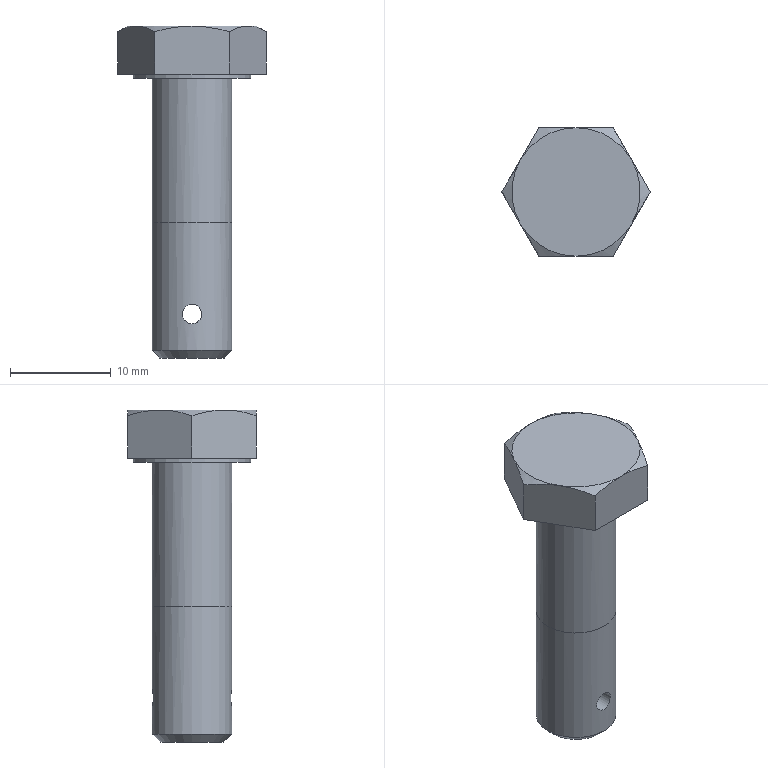Part | NX | features solid 2 | 1 solid | 21 faces | box 14.723 x 12.751 x 32.963 mm | volume 2058 mm3 | plane 10 | cone 7 | cylinder 4 | commonest cylinder face diameters 7.938 x2 1.93 x1 11.684 x1
STEP:
#1=CARTESIAN_POINT('',(0.,-3.969,-29.562));
#2=VERTEX_POINT('',#1);
#3=CARTESIAN_POINT('',(0.7571,-3.91,-29.353));
#4=CARTESIAN_POINT('',(-0.000144,-3.998,-29.667));
#5=CARTESIAN_POINT('',(-0.7565,-3.91,-29.353));
#6=CARTESIAN_POINT('',(-1.07,-3.819,-28.598));
#7=CARTESIAN_POINT('',(-0.7564,-3.91,-27.841));
#8=CARTESIAN_POINT('',(-0.0004429,-3.998,-27.528));
#9=CARTESIAN_POINT('',(0.7557,-3.91,-27.84));
#10=CARTESIAN_POINT('',(1.07,-3.819,-28.597));
#11=CARTESIAN_POINT('',(0.7571,-3.91,-29.353));
#12=CARTESIAN_POINT('',(-0.000144,-3.998,-29.667));
#13=CARTESIAN_POINT('',(-0.7565,-3.91,-29.353));
#14=B_SPLINE_CURVE_WITH_KNOTS('',3,(#3,#4,#5,#6,#7,#8,#9,#10,#11,#12,#13),.UNSPECIFIED.,.T.,.F.,(1,1,1,1,1,1,1,1,1,1,1,1,1,1,1),(-0.002271,-0.001514,-0.0007572,0.,0.0007572,0.001514,0.002271,0.003029,0.003786,0.004543,0.0053,0.006057,0.006814,0.007572,0.008329),.UNSPECIFIED.);
#15=EDGE_CURVE('',#2,#2,#14,.T.);
#16=ORIENTED_EDGE('',*,*,#15,.T.);
#17=EDGE_LOOP('',(#16));
#18=FACE_BOUND('',#17,.T.);
#19=CARTESIAN_POINT('',(-3.969,0.,-19.469));
#20=VERTEX_POINT('',#19);
#21=CARTESIAN_POINT('',(-3.11,3.11,-19.469));
#22=CARTESIAN_POINT('',(-4.398,0.,-19.469));
#23=CARTESIAN_POINT('',(-3.11,-3.11,-19.469));
#24=CARTESIAN_POINT('',(0.,-4.398,-19.469));
#25=CARTESIAN_POINT('',(3.11,-3.11,-19.469));
#26=CARTESIAN_POINT('',(4.398,0.,-19.469));
#27=CARTESIAN_POINT('',(3.11,3.11,-19.469));
#28=CARTESIAN_POINT('',(0.,4.398,-19.469));
#29=CARTESIAN_POINT('',(-3.11,3.11,-19.469));
#30=CARTESIAN_POINT('',(-4.398,0.,-19.469));
#31=CARTESIAN_POINT('',(-3.11,-3.11,-19.469));
#32=B_SPLINE_CURVE_WITH_KNOTS('',3,(#21,#22,#23,#24,#25,#26,#27,#28,#29,#30,#31),.UNSPECIFIED.,.T.,.F.,(1,1,1,1,1,1,1,1,1,1,1,1,1,1,1),(-0.375,-0.25,-0.125,0.,0.125,0.25,0.375,0.5,0.625,0.75,0.875,1.,1.125,1.25,1.375),.UNSPECIFIED.);
#33=EDGE_CURVE('',#20,#20,#32,.T.);
#34=ORIENTED_EDGE('',*,*,#33,.F.);
#35=EDGE_LOOP('',(#34));
#36=FACE_BOUND('',#35,.T.);
#37=CARTESIAN_POINT('',(-3.969,0.,-32.175));
#38=VERTEX_POINT('',#37);
#39=CARTESIAN_POINT('',(0.,0.,-32.175));
#40=DIRECTION('',(0.,0.,-1.));
#41=DIRECTION('',(-1.,0.,0.));
#42=AXIS2_PLACEMENT_3D('',#39,#40,#41);
#43=CIRCLE('',#42,3.969);
#44=EDGE_CURVE('',#38,#38,#43,.T.);
#45=ORIENTED_EDGE('',*,*,#44,.F.);
#46=EDGE_LOOP('',(#45));
#47=FACE_BOUND('',#46,.T.);
#48=CARTESIAN_POINT('',(0.,3.969,-29.562));
#49=VERTEX_POINT('',#48);
#50=CARTESIAN_POINT('',(-0.7571,3.91,-29.353));
#51=CARTESIAN_POINT('',(0.000144,3.998,-29.667));
#52=CARTESIAN_POINT('',(0.7565,3.91,-29.353));
#53=CARTESIAN_POINT('',(1.07,3.819,-28.598));
#54=CARTESIAN_POINT('',(0.7564,3.91,-27.841));
#55=CARTESIAN_POINT('',(0.0004429,3.998,-27.528));
#56=CARTESIAN_POINT('',(-0.7557,3.91,-27.84));
#57=CARTESIAN_POINT('',(-1.07,3.819,-28.597));
#58=CARTESIAN_POINT('',(-0.7571,3.91,-29.353));
#59=CARTESIAN_POINT('',(0.000144,3.998,-29.667));
#60=CARTESIAN_POINT('',(0.7565,3.91,-29.353));
#61=B_SPLINE_CURVE_WITH_KNOTS('',3,(#50,#51,#52,#53,#54,#55,#56,#57,#58,#59,#60),.UNSPECIFIED.,.T.,.F.,(1,1,1,1,1,1,1,1,1,1,1,1,1,1,1),(-0.002271,-0.001514,-0.0007572,0.,0.0007572,0.001514,0.002271,0.003029,0.003786,0.004543,0.0053,0.006057,0.006814,0.007572,0.008329),.UNSPECIFIED.);
#62=EDGE_CURVE('',#49,#49,#61,.T.);
#63=ORIENTED_EDGE('',*,*,#62,.T.);
#64=EDGE_LOOP('',(#63));
#65=FACE_BOUND('',#64,.T.);
#66=CARTESIAN_POINT('',(0.,0.,0.));
#67=DIRECTION('',(0.,0.,-1.));
#68=DIRECTION('',(-1.,0.,0.));
#69=AXIS2_PLACEMENT_3D('',#66,#67,#68);
#70=CYLINDRICAL_SURFACE('',#69,3.969);
#71=ADVANCED_FACE('',(#18,#36,#47,#65),#70,.T.);
#72=CARTESIAN_POINT('',(-3.969,0.,-5.182));
#73=VERTEX_POINT('',#72);
#74=CARTESIAN_POINT('',(0.,0.,-5.182));
#75=DIRECTION('',(0.,0.,-1.));
#76=DIRECTION('',(-1.,0.,0.));
#77=AXIS2_PLACEMENT_3D('',#74,#75,#76);
#78=CIRCLE('',#77,3.969);
#79=EDGE_CURVE('',#73,#73,#78,.T.);
#80=ORIENTED_EDGE('',*,*,#79,.T.);
#81=EDGE_LOOP('',(#80));
#82=FACE_BOUND('',#81,.T.);
#83=ORIENTED_EDGE('',*,*,#33,.T.);
#84=EDGE_LOOP('',(#83));
#85=FACE_BOUND('',#84,.T.);
#86=CARTESIAN_POINT('',(0.,0.,0.));
#87=DIRECTION('',(0.,0.,-1.));
#88=DIRECTION('',(-1.,0.,0.));
#89=AXIS2_PLACEMENT_3D('',#86,#87,#88);
#90=CYLINDRICAL_SURFACE('',#89,3.969);
#91=ADVANCED_FACE('',(#82,#85),#90,.T.);
#92=CARTESIAN_POINT('',(-7.362,0.,-4.775));
#93=VERTEX_POINT('',#92);
#94=CARTESIAN_POINT('',(-3.681,6.375,-4.775));
#95=VERTEX_POINT('',#94);
#96=CARTESIAN_POINT('',(-4.061,5.717,-4.775));
#97=DIRECTION('',(0.5,0.866,0.));
#98=VECTOR('',#97,1000.);
#99=LINE('',#96,#98);
#100=EDGE_CURVE('',#93,#95,#99,.T.);
#101=ORIENTED_EDGE('',*,*,#100,.T.);
#102=CARTESIAN_POINT('',(3.681,6.375,-4.775));
#103=VERTEX_POINT('',#102);
#104=CARTESIAN_POINT('',(5.842,6.375,-4.775));
#105=DIRECTION('',(1.,0.,0.));
#106=VECTOR('',#105,1000.);
#107=LINE('',#104,#106);
#108=EDGE_CURVE('',#95,#103,#107,.T.);
#109=ORIENTED_EDGE('',*,*,#108,.T.);
#110=CARTESIAN_POINT('',(7.362,0.,-4.775));
#111=VERTEX_POINT('',#110);
#112=CARTESIAN_POINT('',(6.982,0.658,-4.775));
#113=DIRECTION('',(0.5,-0.866,0.));
#114=VECTOR('',#113,1000.);
#115=LINE('',#112,#114);
#116=EDGE_CURVE('',#103,#111,#115,.T.);
#117=ORIENTED_EDGE('',*,*,#116,.T.);
#118=CARTESIAN_POINT('',(3.681,-6.375,-4.775));
#119=VERTEX_POINT('',#118);
#120=CARTESIAN_POINT('',(6.982,-0.658,-4.775));
#121=DIRECTION('',(-0.5,-0.866,0.));
#122=VECTOR('',#121,1000.);
#123=LINE('',#120,#122);
#124=EDGE_CURVE('',#111,#119,#123,.T.);
#125=ORIENTED_EDGE('',*,*,#124,.T.);
#126=CARTESIAN_POINT('',(-3.681,-6.375,-4.775));
#127=VERTEX_POINT('',#126);
#128=CARTESIAN_POINT('',(5.842,-6.375,-4.775));
#129=DIRECTION('',(-1.,0.,0.));
#130=VECTOR('',#129,1000.);
#131=LINE('',#128,#130);
#132=EDGE_CURVE('',#119,#127,#131,.T.);
#133=ORIENTED_EDGE('',*,*,#132,.T.);
#134=CARTESIAN_POINT('',(-4.061,-5.717,-4.775));
#135=DIRECTION('',(-0.5,0.866,0.));
#136=VECTOR('',#135,1000.);
#137=LINE('',#134,#136);
#138=EDGE_CURVE('',#127,#93,#137,.T.);
#139=ORIENTED_EDGE('',*,*,#138,.T.);
#140=EDGE_LOOP('',(#101,#109,#117,#125,#133,#139));
#141=FACE_BOUND('',#140,.T.);
#142=CARTESIAN_POINT('',(-5.842,0.,-4.775));
#143=VERTEX_POINT('',#142);
#144=CARTESIAN_POINT('',(0.,0.,-4.775));
#145=DIRECTION('',(0.,0.,-1.));
#146=DIRECTION('',(-1.,0.,0.));
#147=AXIS2_PLACEMENT_3D('',#144,#145,#146);
#148=CIRCLE('',#147,5.842);
#149=EDGE_CURVE('',#143,#143,#148,.T.);
#150=ORIENTED_EDGE('',*,*,#149,.F.);
#151=EDGE_LOOP('',(#150));
#152=FACE_BOUND('',#151,.T.);
#153=CARTESIAN_POINT('',(5.842,0.,-4.775));
#154=DIRECTION('',(0.,0.,-1.));
#155=DIRECTION('',(-1.,0.,0.));
#156=AXIS2_PLACEMENT_3D('',#153,#154,#155);
#157=PLANE('',#156);
#158=ADVANCED_FACE('',(#141,#152),#157,.T.);
#159=CARTESIAN_POINT('',(-3.181,0.,-32.963));
#160=VERTEX_POINT('',#159);
#161=CARTESIAN_POINT('',(0.,0.,-32.963));
#162=DIRECTION('',(0.,0.,-1.));
#163=DIRECTION('',(-1.,0.,0.));
#164=AXIS2_PLACEMENT_3D('',#161,#162,#163);
#165=CIRCLE('',#164,3.181);
#166=EDGE_CURVE('',#160,#160,#165,.T.);
#167=ORIENTED_EDGE('',*,*,#166,.T.);
#168=EDGE_LOOP('',(#167));
#169=FACE_BOUND('',#168,.T.);
#170=CARTESIAN_POINT('',(0.,0.,-32.963));
#171=DIRECTION('',(0.,0.,-1.));
#172=DIRECTION('',(-1.,0.,0.));
#173=AXIS2_PLACEMENT_3D('',#170,#171,#172);
#174=PLANE('',#173);
#175=ADVANCED_FACE('',(#169),#174,.T.);
#176=ORIENTED_EDGE('',*,*,#44,.T.);
#177=EDGE_LOOP('',(#176));
#178=FACE_BOUND('',#177,.T.);
#179=ORIENTED_EDGE('',*,*,#166,.F.);
#180=EDGE_LOOP('',(#179));
#181=FACE_BOUND('',#180,.T.);
#182=CARTESIAN_POINT('',(0.,0.,-32.963));
#183=DIRECTION('',(0.,0.,1.));
#184=DIRECTION('',(1.,0.,0.));
#185=AXIS2_PLACEMENT_3D('',#182,#183,#184);
#186=CONICAL_SURFACE('',#185,3.181,0.7854);
#187=ADVANCED_FACE('',(#178,#181),#186,.T.);
#188=CARTESIAN_POINT('',(-5.842,0.,-5.182));
#189=VERTEX_POINT('',#188);
#190=CARTESIAN_POINT('',(0.,0.,-5.182));
#191=DIRECTION('',(0.,0.,-1.));
#192=DIRECTION('',(-1.,0.,0.));
#193=AXIS2_PLACEMENT_3D('',#190,#191,#192);
#194=CIRCLE('',#193,5.842);
#195=EDGE_CURVE('',#189,#189,#194,.T.);
#196=ORIENTED_EDGE('',*,*,#195,.T.);
#197=EDGE_LOOP('',(#196));
#198=FACE_BOUND('',#197,.T.);
#199=ORIENTED_EDGE('',*,*,#79,.F.);
#200=EDGE_LOOP('',(#199));
#201=FACE_BOUND('',#200,.T.);
#202=CARTESIAN_POINT('',(3.969,0.,-5.182));
#203=DIRECTION('',(0.,0.,-1.));
#204=DIRECTION('',(-1.,0.,0.));
#205=AXIS2_PLACEMENT_3D('',#202,#203,#204);
#206=PLANE('',#205);
#207=ADVANCED_FACE('',(#198,#201),#206,.T.);
#208=ORIENTED_EDGE('',*,*,#149,.T.);
#209=EDGE_LOOP('',(#208));
#210=FACE_BOUND('',#209,.T.);
#211=ORIENTED_EDGE('',*,*,#195,.F.);
#212=EDGE_LOOP('',(#211));
#213=FACE_BOUND('',#212,.T.);
#214=CARTESIAN_POINT('',(0.,0.,0.));
#215=DIRECTION('',(0.,0.,-1.));
#216=DIRECTION('',(-1.,0.,0.));
#217=AXIS2_PLACEMENT_3D('',#214,#215,#216);
#218=CYLINDRICAL_SURFACE('',#217,5.842);
#219=ADVANCED_FACE('',(#210,#213),#218,.T.);
#220=ORIENTED_EDGE('',*,*,#108,.F.);
#221=CARTESIAN_POINT('',(-3.681,6.375,-0.5694));
#222=VERTEX_POINT('',#221);
#223=CARTESIAN_POINT('',(-3.681,6.375,-36.259));
#224=DIRECTION('',(0.,0.,1.));
#225=VECTOR('',#224,1000.);
#226=LINE('',#223,#225);
#227=EDGE_CURVE('',#95,#222,#226,.T.);
#228=ORIENTED_EDGE('',*,*,#227,.T.);
#229=CARTESIAN_POINT('',(0.,6.375,0.));
#230=VERTEX_POINT('',#229);
#231=CARTESIAN_POINT('',(-3.681,6.375,-0.5694));
#232=CARTESIAN_POINT('',(-2.484,6.375,-0.2238));
#233=CARTESIAN_POINT('',(-1.244,6.375,0.));
#234=CARTESIAN_POINT('',(0.,6.375,0.));
#235=B_SPLINE_CURVE_WITH_KNOTS('',3,(#231,#232,#233,#234),.UNSPECIFIED.,.F.,.F.,(4,4),(0.006567,0.01029),.UNSPECIFIED.);
#236=EDGE_CURVE('',#230,#222,#235,.F.);
#237=ORIENTED_EDGE('',*,*,#236,.F.);
#238=CARTESIAN_POINT('',(3.681,6.375,-0.5694));
#239=VERTEX_POINT('',#238);
#240=CARTESIAN_POINT('',(0.,6.375,0.));
#241=CARTESIAN_POINT('',(1.245,6.375,0.));
#242=CARTESIAN_POINT('',(2.49,6.375,-0.2258));
#243=CARTESIAN_POINT('',(3.681,6.375,-0.5694));
#244=B_SPLINE_CURVE_WITH_KNOTS('',3,(#240,#241,#242,#243),.UNSPECIFIED.,.F.,.F.,(4,4),(0.01029,0.01402),.UNSPECIFIED.);
#245=EDGE_CURVE('',#239,#230,#244,.F.);
#246=ORIENTED_EDGE('',*,*,#245,.F.);
#247=CARTESIAN_POINT('',(3.681,6.375,-36.259));
#248=DIRECTION('',(0.,0.,1.));
#249=VECTOR('',#248,1000.);
#250=LINE('',#247,#249);
#251=EDGE_CURVE('',#103,#239,#250,.T.);
#252=ORIENTED_EDGE('',*,*,#251,.F.);
#253=EDGE_LOOP('',(#220,#228,#237,#246,#252));
#254=FACE_BOUND('',#253,.T.);
#255=CARTESIAN_POINT('',(3.681,6.375,-36.259));
#256=DIRECTION('',(0.,1.,0.));
#257=DIRECTION('',(0.,0.,1.));
#258=AXIS2_PLACEMENT_3D('',#255,#256,#257);
#259=PLANE('',#258);
#260=ADVANCED_FACE('',(#254),#259,.T.);
#261=ORIENTED_EDGE('',*,*,#100,.F.);
#262=CARTESIAN_POINT('',(-7.362,0.,-0.5694));
#263=VERTEX_POINT('',#262);
#264=CARTESIAN_POINT('',(-7.362,0.,-36.259));
#265=DIRECTION('',(0.,0.,1.));
#266=VECTOR('',#265,1000.);
#267=LINE('',#264,#266);
#268=EDGE_CURVE('',#93,#263,#267,.T.);
#269=ORIENTED_EDGE('',*,*,#268,.T.);
#270=CARTESIAN_POINT('',(-5.521,3.188,0.));
#271=VERTEX_POINT('',#270);
#272=CARTESIAN_POINT('',(-5.521,3.188,0.));
#273=CARTESIAN_POINT('',(-6.146,2.106,0.));
#274=CARTESIAN_POINT('',(-6.761,1.04,-0.2227));
#275=CARTESIAN_POINT('',(-7.362,0.,-0.5694));
#276=B_SPLINE_CURVE_WITH_KNOTS('',3,(#272,#273,#274,#275),.UNSPECIFIED.,.F.,.F.,(4,4),(0.003725,0.007435),.UNSPECIFIED.);
#277=EDGE_CURVE('',#271,#263,#276,.T.);
#278=ORIENTED_EDGE('',*,*,#277,.F.);
#279=CARTESIAN_POINT('',(-3.681,6.375,-0.5694));
#280=CARTESIAN_POINT('',(-4.283,5.332,-0.2218));
#281=CARTESIAN_POINT('',(-4.894,4.274,0.));
#282=CARTESIAN_POINT('',(-5.521,3.188,0.));
#283=B_SPLINE_CURVE_WITH_KNOTS('',3,(#279,#280,#281,#282),.UNSPECIFIED.,.F.,.F.,(4,4),(0.000000238,0.003725),.UNSPECIFIED.);
#284=EDGE_CURVE('',#222,#271,#283,.T.);
#285=ORIENTED_EDGE('',*,*,#284,.F.);
#286=ORIENTED_EDGE('',*,*,#227,.F.);
#287=EDGE_LOOP('',(#261,#269,#278,#285,#286));
#288=FACE_BOUND('',#287,.T.);
#289=CARTESIAN_POINT('',(-3.681,6.375,-36.259));
#290=DIRECTION('',(-0.866,0.5,0.));
#291=DIRECTION('',(-0.5,-0.866,0.));
#292=AXIS2_PLACEMENT_3D('',#289,#290,#291);
#293=PLANE('',#292);
#294=ADVANCED_FACE('',(#288),#293,.T.);
#295=ORIENTED_EDGE('',*,*,#138,.F.);
#296=CARTESIAN_POINT('',(-3.681,-6.375,-0.5694));
#297=VERTEX_POINT('',#296);
#298=CARTESIAN_POINT('',(-3.681,-6.375,-36.259));
#299=DIRECTION('',(0.,0.,1.));
#300=VECTOR('',#299,1000.);
#301=LINE('',#298,#300);
#302=EDGE_CURVE('',#127,#297,#301,.T.);
#303=ORIENTED_EDGE('',*,*,#302,.T.);
#304=CARTESIAN_POINT('',(-5.521,-3.188,0.));
#305=VERTEX_POINT('',#304);
#306=CARTESIAN_POINT('',(-5.521,-3.188,0.));
#307=CARTESIAN_POINT('',(-4.896,-4.27,0.));
#308=CARTESIAN_POINT('',(-4.281,-5.335,-0.2227));
#309=CARTESIAN_POINT('',(-3.681,-6.375,-0.5694));
#310=B_SPLINE_CURVE_WITH_KNOTS('',3,(#306,#307,#308,#309),.UNSPECIFIED.,.F.,.F.,(4,4),(0.003725,0.007435),.UNSPECIFIED.);
#311=EDGE_CURVE('',#305,#297,#310,.T.);
#312=ORIENTED_EDGE('',*,*,#311,.F.);
#313=CARTESIAN_POINT('',(-7.362,0.,-0.5694));
#314=CARTESIAN_POINT('',(-6.76,-1.043,-0.2218));
#315=CARTESIAN_POINT('',(-6.148,-2.102,0.));
#316=CARTESIAN_POINT('',(-5.521,-3.188,0.));
#317=B_SPLINE_CURVE_WITH_KNOTS('',3,(#313,#314,#315,#316),.UNSPECIFIED.,.F.,.F.,(4,4),(0.000000238,0.003725),.UNSPECIFIED.);
#318=EDGE_CURVE('',#263,#305,#317,.T.);
#319=ORIENTED_EDGE('',*,*,#318,.F.);
#320=ORIENTED_EDGE('',*,*,#268,.F.);
#321=EDGE_LOOP('',(#295,#303,#312,#319,#320));
#322=FACE_BOUND('',#321,.T.);
#323=CARTESIAN_POINT('',(-7.362,0.,-36.259));
#324=DIRECTION('',(-0.866,-0.5,0.));
#325=DIRECTION('',(0.5,-0.866,0.));
#326=AXIS2_PLACEMENT_3D('',#323,#324,#325);
#327=PLANE('',#326);
#328=ADVANCED_FACE('',(#322),#327,.T.);
#329=ORIENTED_EDGE('',*,*,#132,.F.);
#330=CARTESIAN_POINT('',(3.681,-6.375,-0.5694));
#331=VERTEX_POINT('',#330);
#332=CARTESIAN_POINT('',(3.681,-6.375,-36.259));
#333=DIRECTION('',(0.,0.,1.));
#334=VECTOR('',#333,1000.);
#335=LINE('',#332,#334);
#336=EDGE_CURVE('',#119,#331,#335,.T.);
#337=ORIENTED_EDGE('',*,*,#336,.T.);
#338=CARTESIAN_POINT('',(0.,-6.375,0.));
#339=VERTEX_POINT('',#338);
#340=CARTESIAN_POINT('',(0.,-6.375,0.));
#341=CARTESIAN_POINT('',(1.245,-6.375,0.));
#342=CARTESIAN_POINT('',(2.49,-6.375,-0.2258));
#343=CARTESIAN_POINT('',(3.681,-6.375,-0.5694));
#344=B_SPLINE_CURVE_WITH_KNOTS('',3,(#340,#341,#342,#343),.UNSPECIFIED.,.F.,.F.,(4,4),(0.01029,0.01402),.UNSPECIFIED.);
#345=EDGE_CURVE('',#339,#331,#344,.T.);
#346=ORIENTED_EDGE('',*,*,#345,.F.);
#347=CARTESIAN_POINT('',(-3.681,-6.375,-0.5694));
#348=CARTESIAN_POINT('',(-2.484,-6.375,-0.2238));
#349=CARTESIAN_POINT('',(-1.244,-6.375,0.));
#350=CARTESIAN_POINT('',(0.,-6.375,0.));
#351=B_SPLINE_CURVE_WITH_KNOTS('',3,(#347,#348,#349,#350),.UNSPECIFIED.,.F.,.F.,(4,4),(0.006567,0.01029),.UNSPECIFIED.);
#352=EDGE_CURVE('',#297,#339,#351,.T.);
#353=ORIENTED_EDGE('',*,*,#352,.F.);
#354=ORIENTED_EDGE('',*,*,#302,.F.);
#355=EDGE_LOOP('',(#329,#337,#346,#353,#354));
#356=FACE_BOUND('',#355,.T.);
#357=CARTESIAN_POINT('',(-3.681,-6.375,-36.259));
#358=DIRECTION('',(0.,-1.,0.));
#359=DIRECTION('',(0.,0.,-1.));
#360=AXIS2_PLACEMENT_3D('',#357,#358,#359);
#361=PLANE('',#360);
#362=ADVANCED_FACE('',(#356),#361,.T.);
#363=ORIENTED_EDGE('',*,*,#124,.F.);
#364=CARTESIAN_POINT('',(7.362,0.,-0.5694));
#365=VERTEX_POINT('',#364);
#366=CARTESIAN_POINT('',(7.362,0.,-36.259));
#367=DIRECTION('',(0.,0.,1.));
#368=VECTOR('',#367,1000.);
#369=LINE('',#366,#368);
#370=EDGE_CURVE('',#111,#365,#369,.T.);
#371=ORIENTED_EDGE('',*,*,#370,.T.);
#372=CARTESIAN_POINT('',(5.521,-3.188,0.));
#373=VERTEX_POINT('',#372);
#374=CARTESIAN_POINT('',(5.521,-3.188,0.));
#375=CARTESIAN_POINT('',(6.146,-2.106,0.));
#376=CARTESIAN_POINT('',(6.761,-1.04,-0.2227));
#377=CARTESIAN_POINT('',(7.362,0.,-0.5694));
#378=B_SPLINE_CURVE_WITH_KNOTS('',3,(#374,#375,#376,#377),.UNSPECIFIED.,.F.,.F.,(4,4),(0.003725,0.007435),.UNSPECIFIED.);
#379=EDGE_CURVE('',#373,#365,#378,.T.);
#380=ORIENTED_EDGE('',*,*,#379,.F.);
#381=CARTESIAN_POINT('',(3.681,-6.375,-0.5694));
#382=CARTESIAN_POINT('',(4.283,-5.332,-0.2218));
#383=CARTESIAN_POINT('',(4.894,-4.274,0.));
#384=CARTESIAN_POINT('',(5.521,-3.188,0.));
#385=B_SPLINE_CURVE_WITH_KNOTS('',3,(#381,#382,#383,#384),.UNSPECIFIED.,.F.,.F.,(4,4),(0.000000238,0.003725),.UNSPECIFIED.);
#386=EDGE_CURVE('',#331,#373,#385,.T.);
#387=ORIENTED_EDGE('',*,*,#386,.F.);
#388=ORIENTED_EDGE('',*,*,#336,.F.);
#389=EDGE_LOOP('',(#363,#371,#380,#387,#388));
#390=FACE_BOUND('',#389,.T.);
#391=CARTESIAN_POINT('',(3.681,-6.375,-36.259));
#392=DIRECTION('',(0.866,-0.5,0.));
#393=DIRECTION('',(0.5,0.866,0.));
#394=AXIS2_PLACEMENT_3D('',#391,#392,#393);
#395=PLANE('',#394);
#396=ADVANCED_FACE('',(#390),#395,.T.);
#397=ORIENTED_EDGE('',*,*,#116,.F.);
#398=ORIENTED_EDGE('',*,*,#251,.T.);
#399=CARTESIAN_POINT('',(5.521,3.188,0.));
#400=VERTEX_POINT('',#399);
#401=CARTESIAN_POINT('',(5.521,3.188,0.));
#402=CARTESIAN_POINT('',(4.896,4.27,0.));
#403=CARTESIAN_POINT('',(4.281,5.335,-0.2227));
#404=CARTESIAN_POINT('',(3.681,6.375,-0.5694));
#405=B_SPLINE_CURVE_WITH_KNOTS('',3,(#401,#402,#403,#404),.UNSPECIFIED.,.F.,.F.,(4,4),(0.003725,0.007435),.UNSPECIFIED.);
#406=EDGE_CURVE('',#400,#239,#405,.T.);
#407=ORIENTED_EDGE('',*,*,#406,.F.);
#408=CARTESIAN_POINT('',(7.362,0.,-0.5694));
#409=CARTESIAN_POINT('',(6.76,1.043,-0.2218));
#410=CARTESIAN_POINT('',(6.148,2.102,0.));
#411=CARTESIAN_POINT('',(5.521,3.188,0.));
#412=B_SPLINE_CURVE_WITH_KNOTS('',3,(#408,#409,#410,#411),.UNSPECIFIED.,.F.,.F.,(4,4),(0.000000238,0.003725),.UNSPECIFIED.);
#413=EDGE_CURVE('',#365,#400,#412,.T.);
#414=ORIENTED_EDGE('',*,*,#413,.F.);
#415=ORIENTED_EDGE('',*,*,#370,.F.);
#416=EDGE_LOOP('',(#397,#398,#407,#414,#415));
#417=FACE_BOUND('',#416,.T.);
#418=CARTESIAN_POINT('',(7.362,0.,-36.259));
#419=DIRECTION('',(0.866,0.5,0.));
#420=DIRECTION('',(-0.5,0.866,0.));
#421=AXIS2_PLACEMENT_3D('',#418,#419,#420);
#422=PLANE('',#421);
#423=ADVANCED_FACE('',(#417),#422,.T.);
#424=CARTESIAN_POINT('',(0.,0.,0.));
#425=DIRECTION('',(0.,0.,-1.));
#426=DIRECTION('',(-1.,0.,0.));
#427=AXIS2_PLACEMENT_3D('',#424,#425,#426);
#428=CIRCLE('',#427,6.375);
#429=EDGE_CURVE('',#400,#373,#428,.T.);
#430=ORIENTED_EDGE('',*,*,#429,.T.);
#431=ORIENTED_EDGE('',*,*,#379,.T.);
#432=ORIENTED_EDGE('',*,*,#413,.T.);
#433=EDGE_LOOP('',(#430,#431,#432));
#434=FACE_BOUND('',#433,.T.);
#435=CARTESIAN_POINT('',(0.,0.,-0.5719));
#436=DIRECTION('',(0.,0.,-1.));
#437=DIRECTION('',(-1.,0.,0.));
#438=AXIS2_PLACEMENT_3D('',#435,#436,#437);
#439=CONICAL_SURFACE('',#438,7.366,1.047);
#440=ADVANCED_FACE('',(#434),#439,.T.);
#441=CARTESIAN_POINT('',(0.,0.,0.));
#442=DIRECTION('',(0.,0.,-1.));
#443=DIRECTION('',(-1.,0.,0.));
#444=AXIS2_PLACEMENT_3D('',#441,#442,#443);
#445=CIRCLE('',#444,6.375);
#446=EDGE_CURVE('',#373,#339,#445,.T.);
#447=ORIENTED_EDGE('',*,*,#446,.T.);
#448=ORIENTED_EDGE('',*,*,#345,.T.);
#449=ORIENTED_EDGE('',*,*,#386,.T.);
#450=EDGE_LOOP('',(#447,#448,#449));
#451=FACE_BOUND('',#450,.T.);
#452=CARTESIAN_POINT('',(0.,0.,-0.5719));
#453=DIRECTION('',(0.,0.,-1.));
#454=DIRECTION('',(-1.,0.,0.));
#455=AXIS2_PLACEMENT_3D('',#452,#453,#454);
#456=CONICAL_SURFACE('',#455,7.366,1.047);
#457=ADVANCED_FACE('',(#451),#456,.T.);
#458=CARTESIAN_POINT('',(0.,0.,0.));
#459=DIRECTION('',(0.,0.,-1.));
#460=DIRECTION('',(-1.,0.,0.));
#461=AXIS2_PLACEMENT_3D('',#458,#459,#460);
#462=CIRCLE('',#461,6.375);
#463=EDGE_CURVE('',#339,#305,#462,.T.);
#464=ORIENTED_EDGE('',*,*,#463,.T.);
#465=ORIENTED_EDGE('',*,*,#311,.T.);
#466=ORIENTED_EDGE('',*,*,#352,.T.);
#467=EDGE_LOOP('',(#464,#465,#466));
#468=FACE_BOUND('',#467,.T.);
#469=CARTESIAN_POINT('',(0.,0.,-0.5719));
#470=DIRECTION('',(0.,0.,-1.));
#471=DIRECTION('',(-1.,0.,0.));
#472=AXIS2_PLACEMENT_3D('',#469,#470,#471);
#473=CONICAL_SURFACE('',#472,7.366,1.047);
#474=ADVANCED_FACE('',(#468),#473,.T.);
#475=CARTESIAN_POINT('',(0.,0.,0.));
#476=DIRECTION('',(0.,0.,-1.));
#477=DIRECTION('',(-1.,0.,0.));
#478=AXIS2_PLACEMENT_3D('',#475,#476,#477);
#479=CIRCLE('',#478,6.375);
#480=EDGE_CURVE('',#305,#271,#479,.T.);
#481=ORIENTED_EDGE('',*,*,#480,.T.);
#482=ORIENTED_EDGE('',*,*,#277,.T.);
#483=ORIENTED_EDGE('',*,*,#318,.T.);
#484=EDGE_LOOP('',(#481,#482,#483));
#485=FACE_BOUND('',#484,.T.);
#486=CARTESIAN_POINT('',(0.,0.,-0.5719));
#487=DIRECTION('',(0.,0.,-1.));
#488=DIRECTION('',(-1.,0.,0.));
#489=AXIS2_PLACEMENT_3D('',#486,#487,#488);
#490=CONICAL_SURFACE('',#489,7.366,1.047);
#491=ADVANCED_FACE('',(#485),#490,.T.);
#492=CARTESIAN_POINT('',(0.,0.,0.));
#493=DIRECTION('',(0.,0.,-1.));
#494=DIRECTION('',(-1.,0.,0.));
#495=AXIS2_PLACEMENT_3D('',#492,#493,#494);
#496=CIRCLE('',#495,6.375);
#497=EDGE_CURVE('',#271,#230,#496,.T.);
#498=ORIENTED_EDGE('',*,*,#497,.T.);
#499=ORIENTED_EDGE('',*,*,#236,.T.);
#500=ORIENTED_EDGE('',*,*,#284,.T.);
#501=EDGE_LOOP('',(#498,#499,#500));
#502=FACE_BOUND('',#501,.T.);
#503=CARTESIAN_POINT('',(0.,0.,-0.5719));
#504=DIRECTION('',(0.,0.,-1.));
#505=DIRECTION('',(-1.,0.,0.));
#506=AXIS2_PLACEMENT_3D('',#503,#504,#505);
#507=CONICAL_SURFACE('',#506,7.366,1.047);
#508=ADVANCED_FACE('',(#502),#507,.T.);
#509=ORIENTED_EDGE('',*,*,#497,.F.);
#510=ORIENTED_EDGE('',*,*,#480,.F.);
#511=ORIENTED_EDGE('',*,*,#463,.F.);
#512=ORIENTED_EDGE('',*,*,#446,.F.);
#513=ORIENTED_EDGE('',*,*,#429,.F.);
#514=CARTESIAN_POINT('',(0.,0.,0.));
#515=DIRECTION('',(0.,0.,-1.));
#516=DIRECTION('',(-1.,0.,0.));
#517=AXIS2_PLACEMENT_3D('',#514,#515,#516);
#518=CIRCLE('',#517,6.375);
#519=EDGE_CURVE('',#230,#400,#518,.T.);
#520=ORIENTED_EDGE('',*,*,#519,.F.);
#521=EDGE_LOOP('',(#509,#510,#511,#512,#513,#520));
#522=FACE_BOUND('',#521,.T.);
#523=CARTESIAN_POINT('',(6.375,0.,0.));
#524=DIRECTION('',(0.,0.,1.));
#525=DIRECTION('',(1.,0.,0.));
#526=AXIS2_PLACEMENT_3D('',#523,#524,#525);
#527=PLANE('',#526);
#528=ADVANCED_FACE('',(#522),#527,.T.);
#529=ORIENTED_EDGE('',*,*,#406,.T.);
#530=ORIENTED_EDGE('',*,*,#245,.T.);
#531=ORIENTED_EDGE('',*,*,#519,.T.);
#532=EDGE_LOOP('',(#529,#530,#531));
#533=FACE_BOUND('',#532,.T.);
#534=CARTESIAN_POINT('',(0.,0.,-0.5719));
#535=DIRECTION('',(0.,0.,-1.));
#536=DIRECTION('',(-1.,0.,0.));
#537=AXIS2_PLACEMENT_3D('',#534,#535,#536);
#538=CONICAL_SURFACE('',#537,7.366,1.047);
#539=ADVANCED_FACE('',(#533),#538,.T.);
#540=ORIENTED_EDGE('',*,*,#62,.F.);
#541=EDGE_LOOP('',(#540));
#542=FACE_BOUND('',#541,.T.);
#543=ORIENTED_EDGE('',*,*,#15,.F.);
#544=EDGE_LOOP('',(#543));
#545=FACE_BOUND('',#544,.T.);
#546=CARTESIAN_POINT('',(0.,7.013,-28.597));
#547=DIRECTION('',(0.,-1.,0.));
#548=DIRECTION('',(0.,0.,-1.));
#549=AXIS2_PLACEMENT_3D('',#546,#547,#548);
#550=CYLINDRICAL_SURFACE('',#549,0.9652);
#551=ADVANCED_FACE('',(#542,#545),#550,.F.);
#552=CLOSED_SHELL('',(#71,#91,#158,#175,#187,#207,#219,#260,#294,#328,#362,#396,#423,#440,#457,#474,#491,#508,#528,#539,#551));
#553=MANIFOLD_SOLID_BREP('',#552);
#554=(LENGTH_UNIT()NAMED_UNIT(*)SI_UNIT(.MILLI.,.METRE.));
#555=UNCERTAINTY_MEASURE_WITH_UNIT(LENGTH_MEASURE(0.0508),#554,'','');
#556=(NAMED_UNIT(*)PLANE_ANGLE_UNIT()SI_UNIT($,.RADIAN.));
#557=(NAMED_UNIT(*)SI_UNIT($,.STERADIAN.)SOLID_ANGLE_UNIT());
#558=(GEOMETRIC_REPRESENTATION_CONTEXT(3)GLOBAL_UNCERTAINTY_ASSIGNED_CONTEXT((#555))GLOBAL_UNIT_ASSIGNED_CONTEXT((#554,#556,#557))REPRESENTATION_CONTEXT('',''));
#559=ADVANCED_BREP_SHAPE_REPRESENTATION('',(#553),#558);